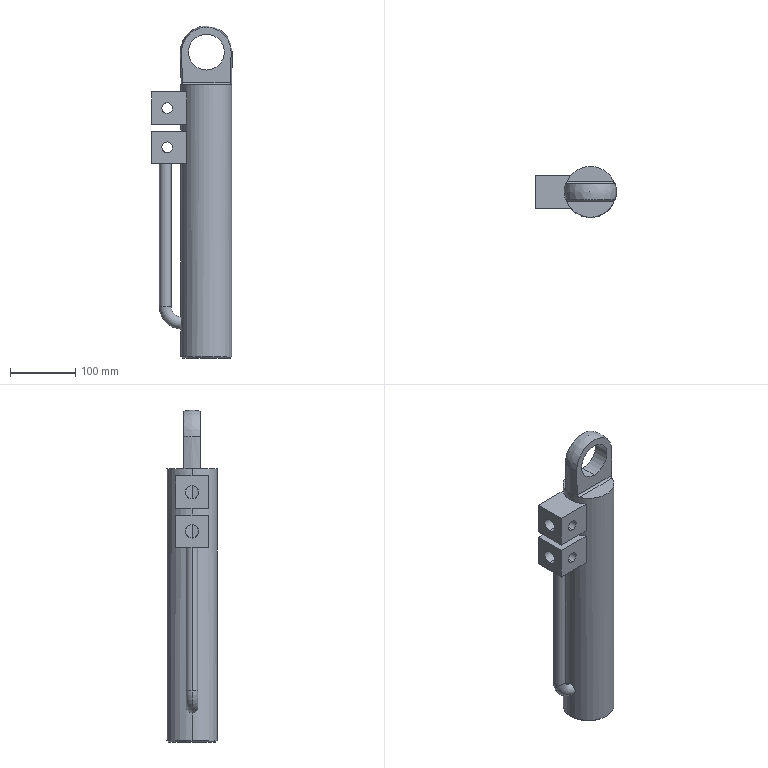Part | SolidWorks | features ICE 5, HoleWzd 2, RevCut 2, Chamfer 1, Extrusion 1, Fillet 1, MirrorPattern 1, Sweep 1 | 1 solid | 59 faces | box 124 x 78 x 509 mm | volume 1078781 mm3 | cylinder 30 | plane 19 | torus 4 | cone 2 | sphere 2 | spline 2 | commonest cylinder face diameters 16.5 x8 10 x4 20.5 x4 78 x4 6 x2 18 x2